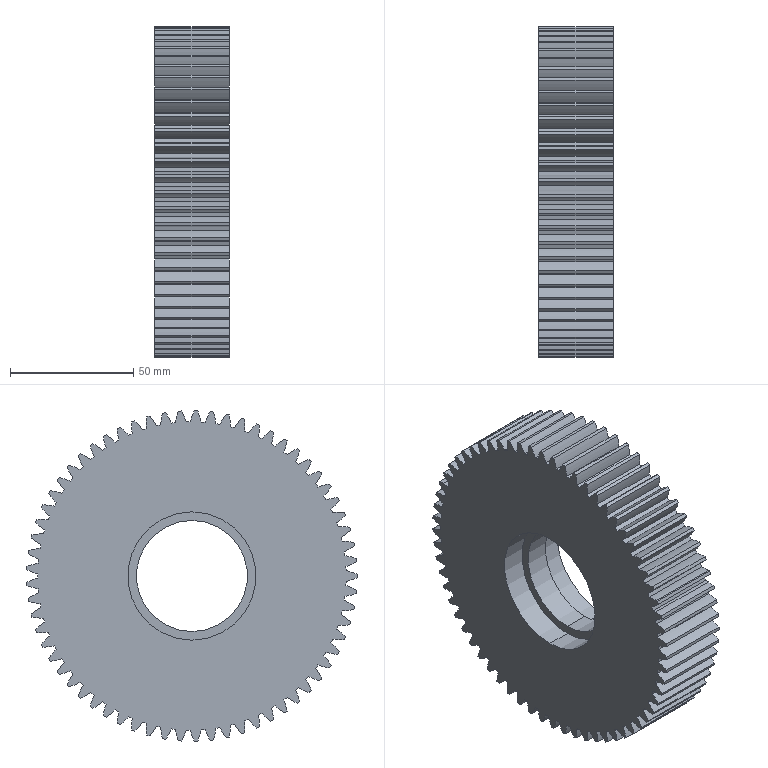Part | SolidWorks | features ICE 2, MBimport 1, MirrorPattern 1 | 1 solid | 274 faces | box 30 x 133.951 x 133.986 mm | volume 336105 mm3 | cylinder 270 | plane 4 | commonest cylinder face diameters 52 x138 124.998 x65 134 x65 45 x2